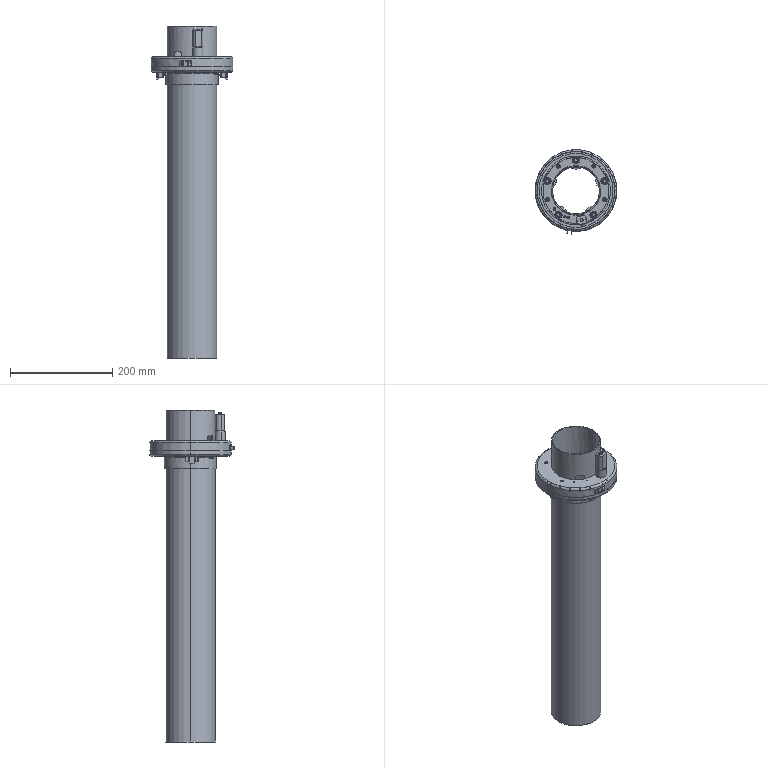Part | SolidWorks | features InContextFeatHolder 5, ReferencePattern 4, LocalCirPattern 1 | 18 solids | 3387 faces | volume 425730 mm3 | plane 1544 | cylinder 1352 | spline 370 | torus 87 | cone 25 | sphere 9 | commonest cylinder face diameters 6.3 x514 0.95 x144 128.755 x105 134.375 x105 15 x66 9.375 x60